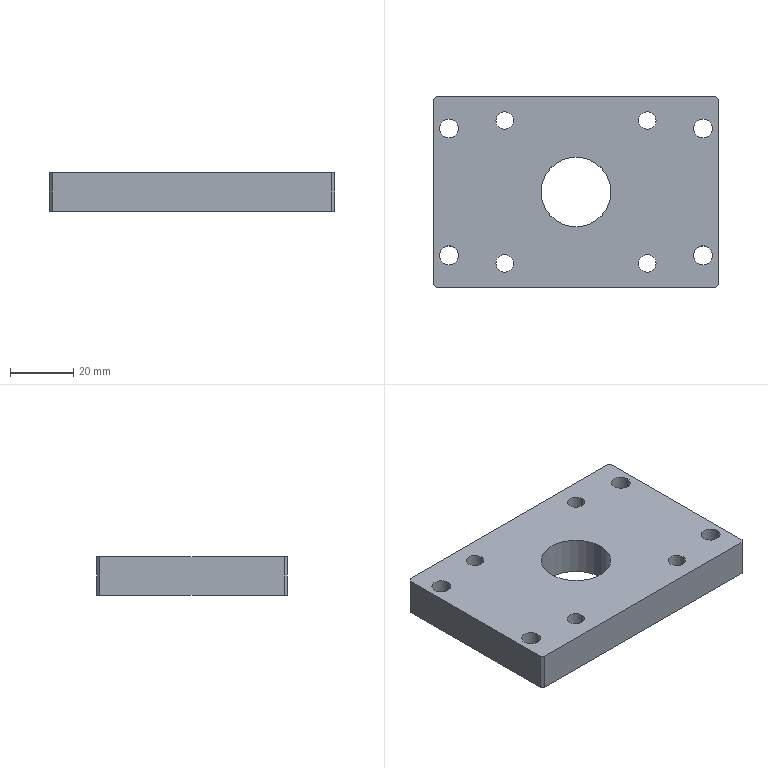Part | STEP file | PN_0004 Plate 4_Default | 1 solid | 48 faces | box 90 x 60 x 12 mm | volume 56425 mm3 | cylinder 30 | plane 14 | cone 4 | commonest cylinder face diameters 5.5 x8 6 x8 9.5 x8 4 x4 22 x2